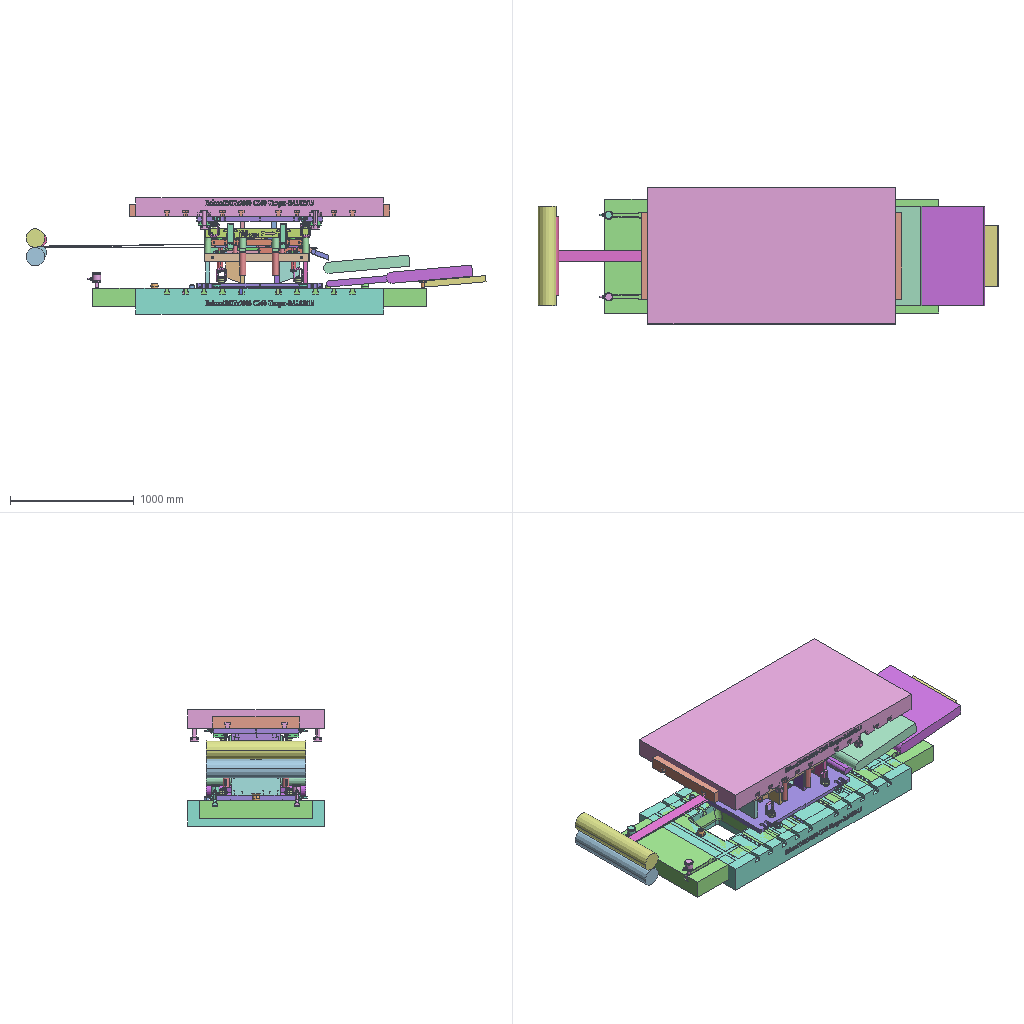Assembly | CATIA | 131 different items | 328 placed | box 3716 x 1100 x 940 mm
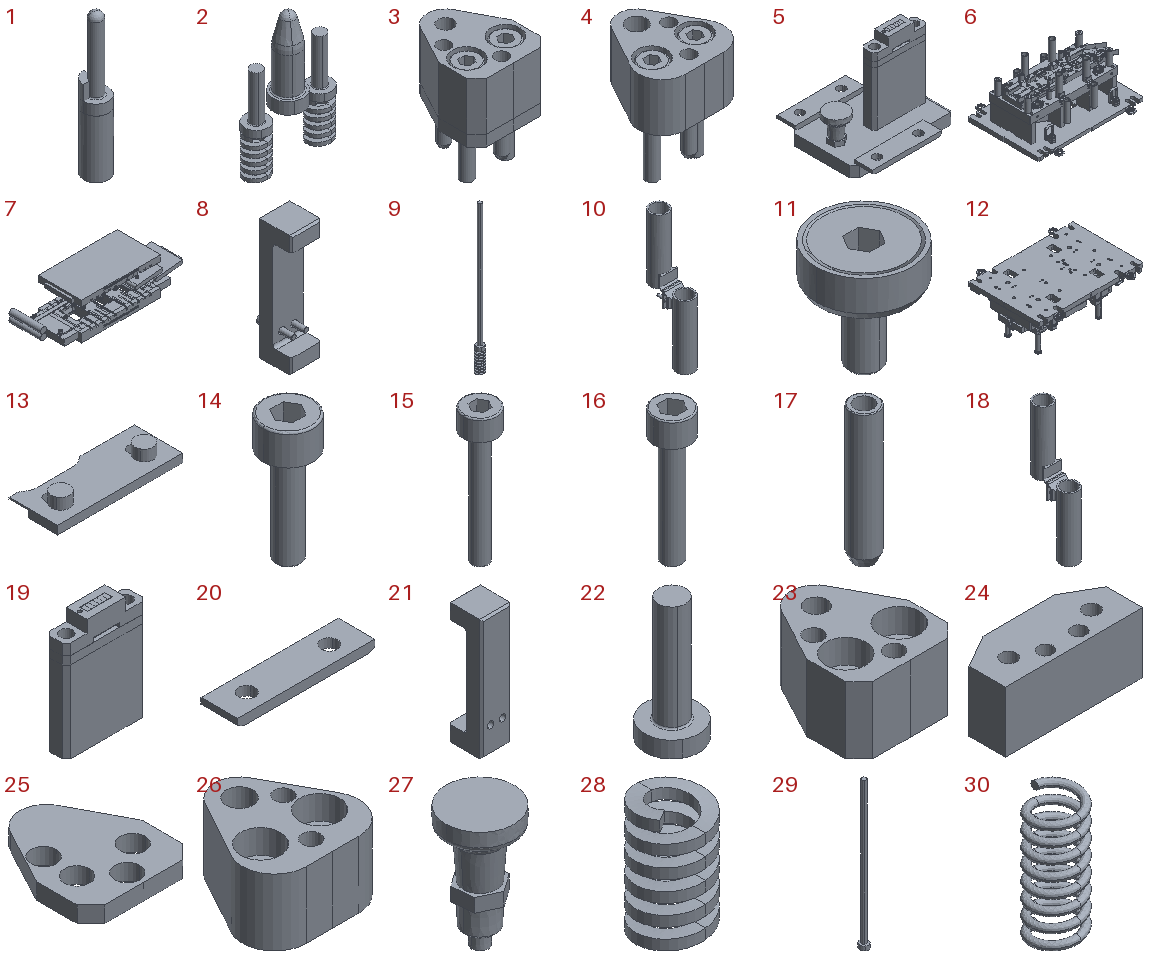Parts list (item | name | quantity | parent item | size | volume):
1 | (subassembly) | x1 | in 6 | 12 x 12 x 68 mm | 4157 mm3
2 | (subassembly) | x7 | in 12 | 37 x 13 x 54.5 mm | 4509 mm3
3 | (subassembly) | x1 | in 12 | 38 x 44.5 x 54 mm | 36944 mm3
4 | (subassembly) | x1 | in 12 | 43.7 x 44.5 x 54 mm | 31784 mm3
5 | (subassembly) | x1 | in 12 | 108 x 104 x 97.9 mm | 166233 mm3
6 | (subassembly) | x1 | - | - | 67388913 mm3
7 | (subassembly) | x1 | - | - | 1311212838 mm3
8 | (subassembly) | x4 | in 12 | 50 x 65 x 200 mm | 324981 mm3
9 | (subassembly) | x3 | in 12 | 6.75 x 6.75 x 120 mm | 905.182 mm3
10 | (subassembly) | x4 | in 6 | 51 x 127 x 364.6 mm | 245023 mm3
11 | (subassembly) | x4 | in 6 | 14 x 14 x 16 mm | 880.628 mm3
12 | (subassembly) | x1 | - | - | 70681805 mm3
13 | - | x1 | in 6 | 90 x 35 x 14 mm | 17820 mm3
14 | - | x8 | in 10 | 13 x 13 x 33 mm | 1675 mm3
15 | - | x4 | in 3, 4 | 13 x 13 x 53 mm | 2318 mm3
16 | - | x8 | in 8 | 15 x 15 x 55 mm | 3637 mm3
17 | - | x4 | in 3, 4 | 6 x 6 x 30 mm | 692.749 mm3
18 | - | x4 | in 10 | 51 x 127 x 364.6 mm | 241674 mm3
19 | - | x1 | in 5 | 58 x 15 x 81.9 mm | 59314 mm3
20 | - | x2 | in 5 | 75 x 20 x 5 mm | 6760 mm3
21 | - | x4 | in 8 | 50 x 55 x 200 mm | 317707 mm3
22 | - | x14 | in 2 | 10 x 10 x 22.5 mm | 618.813 mm3
23 | - | x1 | in 3 | 38 x 44.5 x 25 mm | 24726 mm3
24 | - | x1 | in 6 | 75 x 30 x 33 mm | 61014 mm3
25 | - | x1 | in 3 | 38 x 44.5 x 5.8 mm | 6197 mm3
26 | - | x1 | in 4 | 43.7 x 44.5 x 25 mm | 25763 mm3
27 | - | x1 | in 5 | 25 x 25 x 45 mm | 8256 mm3
28 | - | x14 | in 2 | 9.8 x 9.8 x 17.5 mm | 377.238 mm3
29 | - | x3 | in 9 | 6 x 6 x 103 mm | 791.681 mm3
30 | - | x3 | in 9 | 6.75 x 6.75 x 17 mm | 113.5 mm3
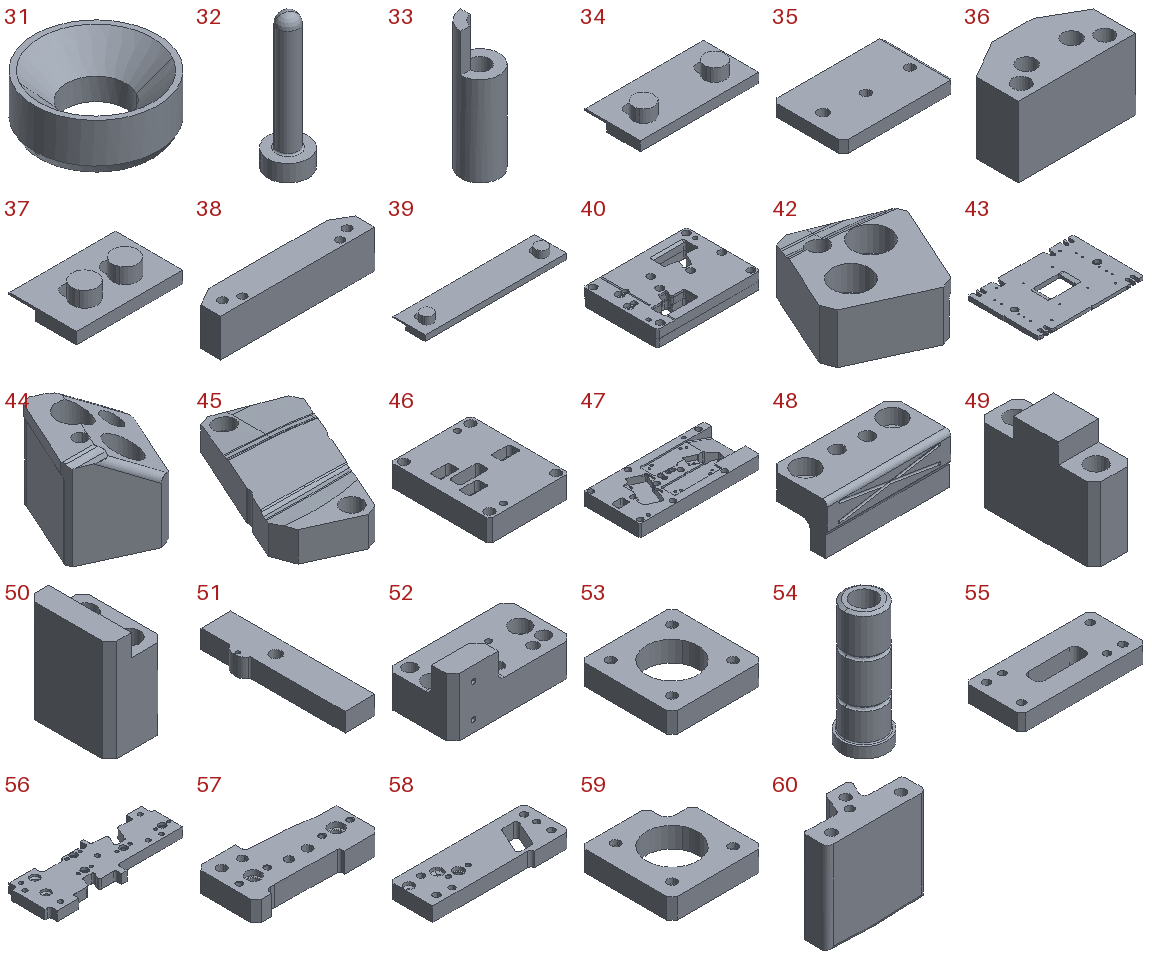31 | - | x4 | in 11 | 14 x 14 x 5.5 mm | 510.162 mm3
32 | - | x1 | in 1 | 12 x 12 x 40 mm | 1528 mm3
33 | - | x1 | in 1 | 12 x 12 x 40 mm | 2630 mm3
34 | - | x1 | in 6 | 75 x 35 x 14 mm | 15567 mm3
35 | - | x1 | in 5 | 108 x 70 x 11.8 mm | 85144 mm3
36 | - | x1 | in 6 | 55 x 30 x 33 mm | 41214 mm3
37 | - | x1 | in 6 | 55 x 35 x 14 mm | 11367 mm3
38 | - | x2 | in 6 | 155 x 30 x 38 mm | 161459 mm3
39 | - | x2 | in 6 | 155 x 35 x 14 mm | 32367 mm3
40 | - | x1 | in 6 | 267 x 192 x 42 mm | 1738037 mm3
41 | - | x1 | in 6 | - | -
42 | - | x1 | in 6 | 50.331 x 51.489 x 20 mm | 26197 mm3
43 | - | x1 | in 6 | 1020 x 690 x 40 mm | 24770735 mm3
44 | - | x1 | in 6 | 49.997 x 51.489 x 42 mm | 42846 mm3
45 | - | x1 | in 6 | 93.337 x 126.037 x 22 mm | 134150 mm3
46 | - | x1 | in 6 | 155 x 192 x 42 mm | 1025287 mm3
47 | - | x1 | in 6 | 406 x 192 x 42 mm | 2564090 mm3
48 | - | x2 | in 6 | 74 x 35 x 30 mm | 43302 mm3
49 | - | x1 | in 6 | 18 x 52 x 42 mm | 29335 mm3
50 | - | x1 | in 6 | 23 x 34 x 42 mm | 23686 mm3
51 | - | x1 | in 6 | 19 x 77 x 10 mm | 12253 mm3
52 | - | x1 | in 6 | 93 x 51 x 45 mm | 117179 mm3
53 | - | x3 | in 12 | 90 x 90 x 20 mm | 109855 mm3
54 | - | x7 | in 6 | 21 x 21 x 57 mm | 12762 mm3
55 | - | x1 | in 12 | 150 x 68 x 19.5 mm | 164563 mm3
56 | - | x1 | in 12 | 290 x 100 x 19.5 mm | 379711 mm3
57 | - | x1 | in 12 | 120 x 58 x 19.5 mm | 94988 mm3
58 | - | x1 | in 12 | 183 x 63 x 19.5 mm | 178829 mm3
59 | - | x1 | in 12 | 90 x 90 x 20 mm | 102848 mm3
60 | - | x1 | in 12 | 87 x 41 x 82 mm | 179725 mm3
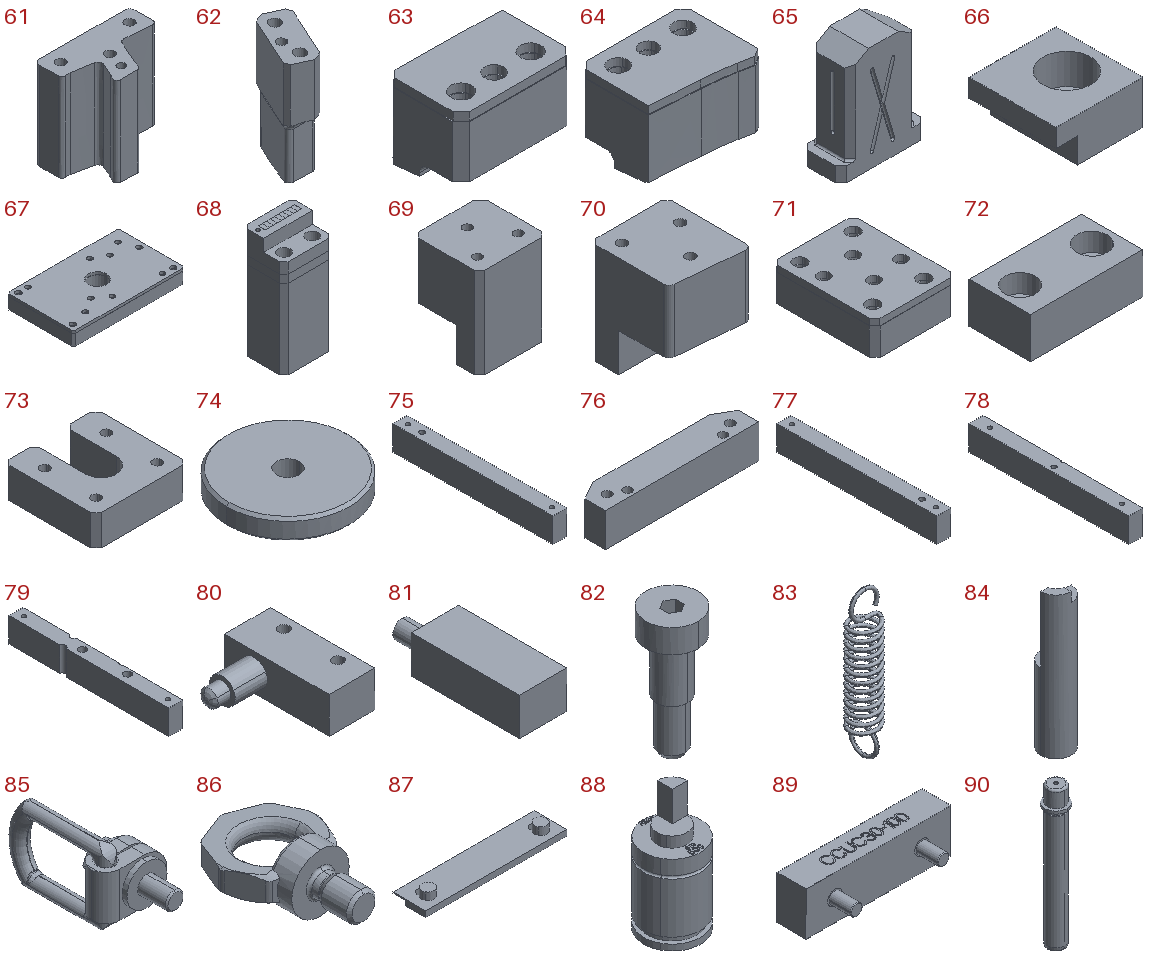61 | - | x1 | in 12 | 87 x 53 x 82 mm | 218758 mm3
62 | - | x1 | in 12 | 38.266 x 50.474 x 82 mm | 71988 mm3
63 | - | x1 | in 12 | 66 x 43.369 x 43.322 mm | 92205 mm3
64 | - | x1 | in 12 | 67 x 51.664 x 44.519 mm | 110677 mm3
65 | - | x3 | in 6 | 46 x 21 x 57 mm | 41695 mm3
66 | - | x24 | in 6, 12 | 20 x 20 x 10 mm | 2655 mm3
67 | - | x1 | in 12 | 250 x 150 x 30.8 mm | 950140 mm3
68 | - | x1 | in 12 | 36 x 30 x 81.8 mm | 74943 mm3
69 | - | x1 | in 12 | 66 x 65 x 89 mm | 271119 mm3
70 | - | x1 | in 12 | 67 x 74.702 x 89 mm | 308137 mm3
71 | - | x1 | in 12 | 75 x 95 x 30.8 mm | 163916 mm3
72 | - | x8 | in 12 | 55 x 30 x 20 mm | 28420 mm3
73 | - | x4 | in 12 | 90 x 90 x 30 mm | 170727 mm3
74 | - | x4 | in 12 | 48 x 48 x 8 mm | 13819 mm3
75 | - | x1 | in 12 | 35 x 400 x 61.7 mm | 838529 mm3
76 | - | x2 | in 6 | 150 x 30 x 33 mm | 135264 mm3
77 | - | x1 | in 12 | 35 x 400 x 61.7 mm | 838590 mm3
78 | - | x1 | in 12 | 35 x 400 x 61.7 mm | 841945 mm3
79 | - | x1 | in 12 | 35 x 400 x 61.7 mm | 807204 mm3
80 | - | x1 | in 6 | 44.5 x 49 x 17 mm | 19294 mm3
81 | - | x1 | in 6 | 21.5 x 61 x 17 mm | 18577 mm3
82 | - | x2 | in 6 | 10 x 10 x 24 mm | 794.336 mm3
83 | - | x1 | in 6 | 8 x 8 x 40.5 mm | 205.926 mm3
84 | - | x13 | in 6 | 16 x 16 x 75 mm | 8482 mm3
85 | - | x8 | in 6, 12 | 69 x 158.5 x 82 mm | 178228 mm3
86 | - | x8 | in 6, 12 | 66.676 x 99.338 x 40 mm | 54798 mm3
87 | - | x2 | in 6 | 150 x 35 x 14 mm | 31317 mm3
88 | - | x6 | in 12 | 38 x 38 x 80 mm | 62160 mm3
89 | - | x4 | in 12 | 100 x 35 x 30 mm | 56836 mm3
90 | - | x4 | in 12 | 50 x 50 x 317 mm | 398728 mm3
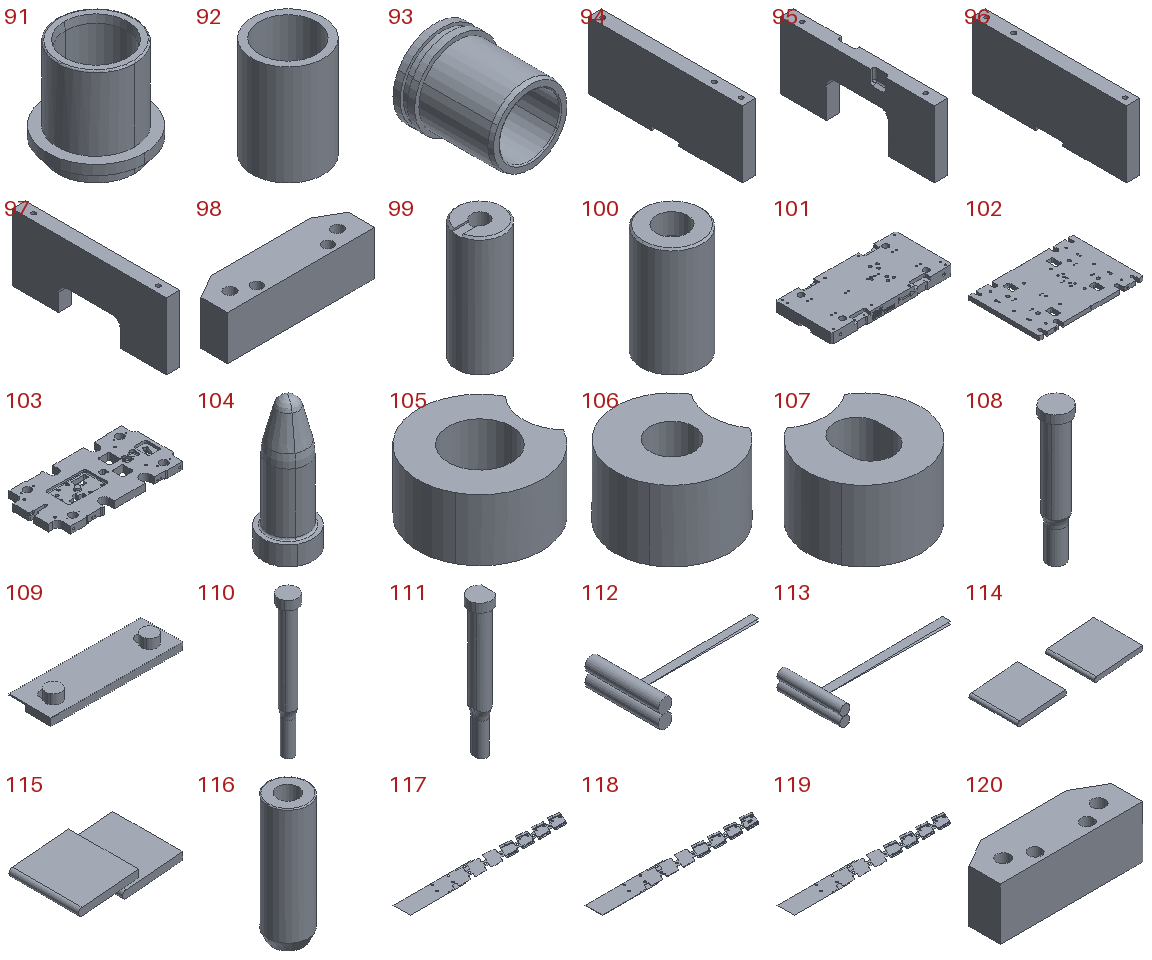91 | - | x4 | in 12 | 63 x 63 x 63 mm | 51378 mm3
92 | - | x4 | in 6 | 50 x 50 x 70.6 mm | 49904 mm3
93 | - | x4 | in 6 | 70 x 79 x 70 mm | 99847 mm3
94 | - | x1 | in 6 | 35 x 400 x 173 mm | 2372229 mm3
95 | - | x1 | in 6 | 35 x 400 x 173 mm | 1827940 mm3
96 | - | x1 | in 6 | 35 x 400 x 173 mm | 2372229 mm3
97 | - | x1 | in 6 | 35 x 400 x 173 mm | 2052248 mm3
98 | - | x1 | in 6 | 110 x 30 x 33 mm | 95664 mm3
99 | - | x4 | in 6 | 50 x 50 x 125.3 mm | 227926 mm3
100 | - | x4 | in 6 | 35 x 35 x 63 mm | 52659 mm3
101 | - | x1 | in 12 | 850 x 401 x 70 mm | 21718763 mm3
102 | - | x1 | in 12 | 1020 x 690 x 40 mm | 26113969 mm3
103 | - | x1 | in 12 | 810 x 400 x 45 mm | 9884776 mm3
104 | - | x7 | in 2 | 13 x 13 x 34 mm | 2517 mm3
105 | - | x2 | in 6 | 20 x 20 x 10 mm | 2190 mm3
106 | - | x1 | in 6 | 16 x 16 x 10 mm | 1611 mm3
107 | - | x1 | in 6 | 16 x 16 x 10 mm | 1487 mm3
108 | - | x2 | in 12 | 16 x 16 x 82.2 mm | 9788 mm3
109 | - | x1 | in 6 | 110 x 35 x 14 mm | 22917 mm3
110 | - | x1 | in 12 | 11 x 11 x 81.7 mm | 3799 mm3
111 | - | x1 | in 12 | 11.5 x 13 x 82.2 mm | 5687 mm3
112 | - | x1 | in 7 | 1458 x 800 x 300 mm | 28421278 mm3
113 | - | x1 | in 7 | 1390 x 632 x 200 mm | 10069805 mm3
114 | - | x1 | in 7 | 1288 x 500 x 91.304 mm | 24731748 mm3
115 | - | x1 | in 7 | 1204 x 800 x 226.48 mm | 98689379 mm3
116 | - | x2 | in 6 | 8 x 8 x 25 mm | 1095 mm3
117 | - | x1 | in 7 | - | -
118 | - | x1 | in 7 | - | 50816 mm3
119 | - | x1 | in 7 | - | -
120 | - | x1 | in 6 | 90 x 30 x 33 mm | 75864 mm3
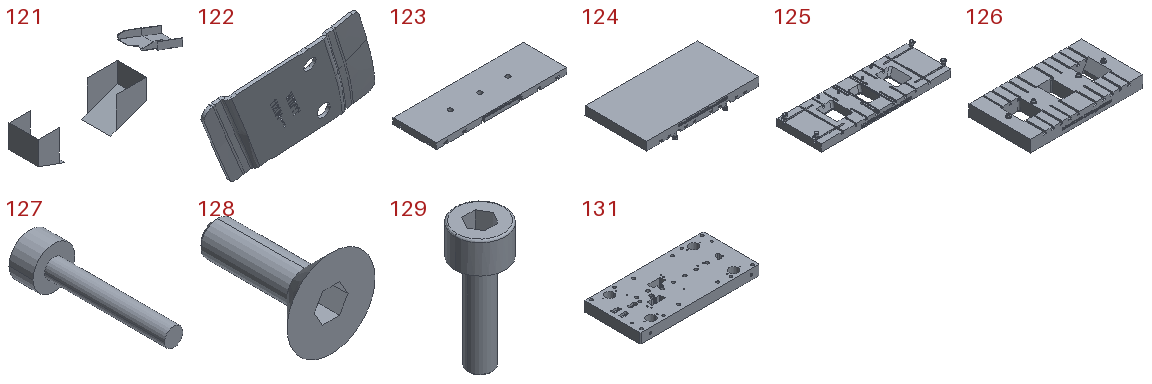121 | - | x1 | in 6 | 830.623 x 160 x 315 mm | 5795629 mm3
122 | - | x1 | in 7 | 99.513 x 15.41 x 56.212 mm | 6324 mm3
123 | - | x1 | in 7 | 2100 x 700 x 95 mm | 132752319 mm3
124 | - | x1 | in 7 | 2000 x 1100 x 259.5 mm | 317583648 mm3
125 | - | x1 | in 7 | - | 311750025 mm3
126 | - | x1 | in 7 | 2000 x 1100 x 250 mm | 378251028 mm3
127 | - | x2 | in 6 | 7 x 24 x 7 mm | 304.892 mm3
128 | - | x4 | in 11 | 12 x 16 x 12 mm | 370.466 mm3
129 | - | x4 | in 12 | 13 x 13 x 33 mm | 1675 mm3
130 | - | x1 | in 1 | - | -
131 | - | x1 | in 6 | 850 x 400 x 70 mm | 21665405 mm3